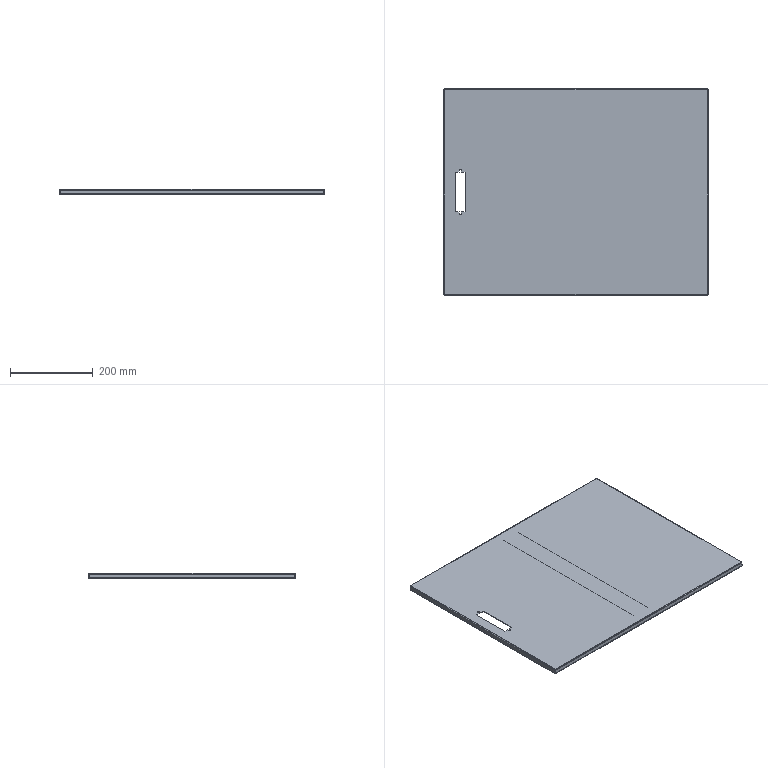Part | SolidWorks | features BaseBody 2 | 2 solids | 96 faces | box 641 x 500 x 13 mm | volume 603273 mm3 | plane 58 | cylinder 22 | spline 16 | commonest cylinder face diameters 1.473 x10 4.473 x10 6 x2